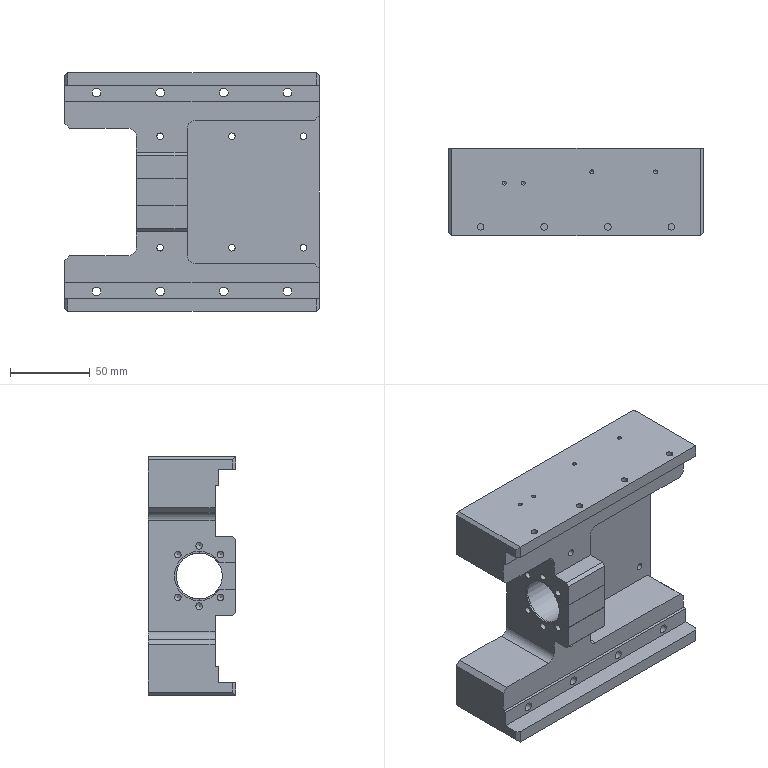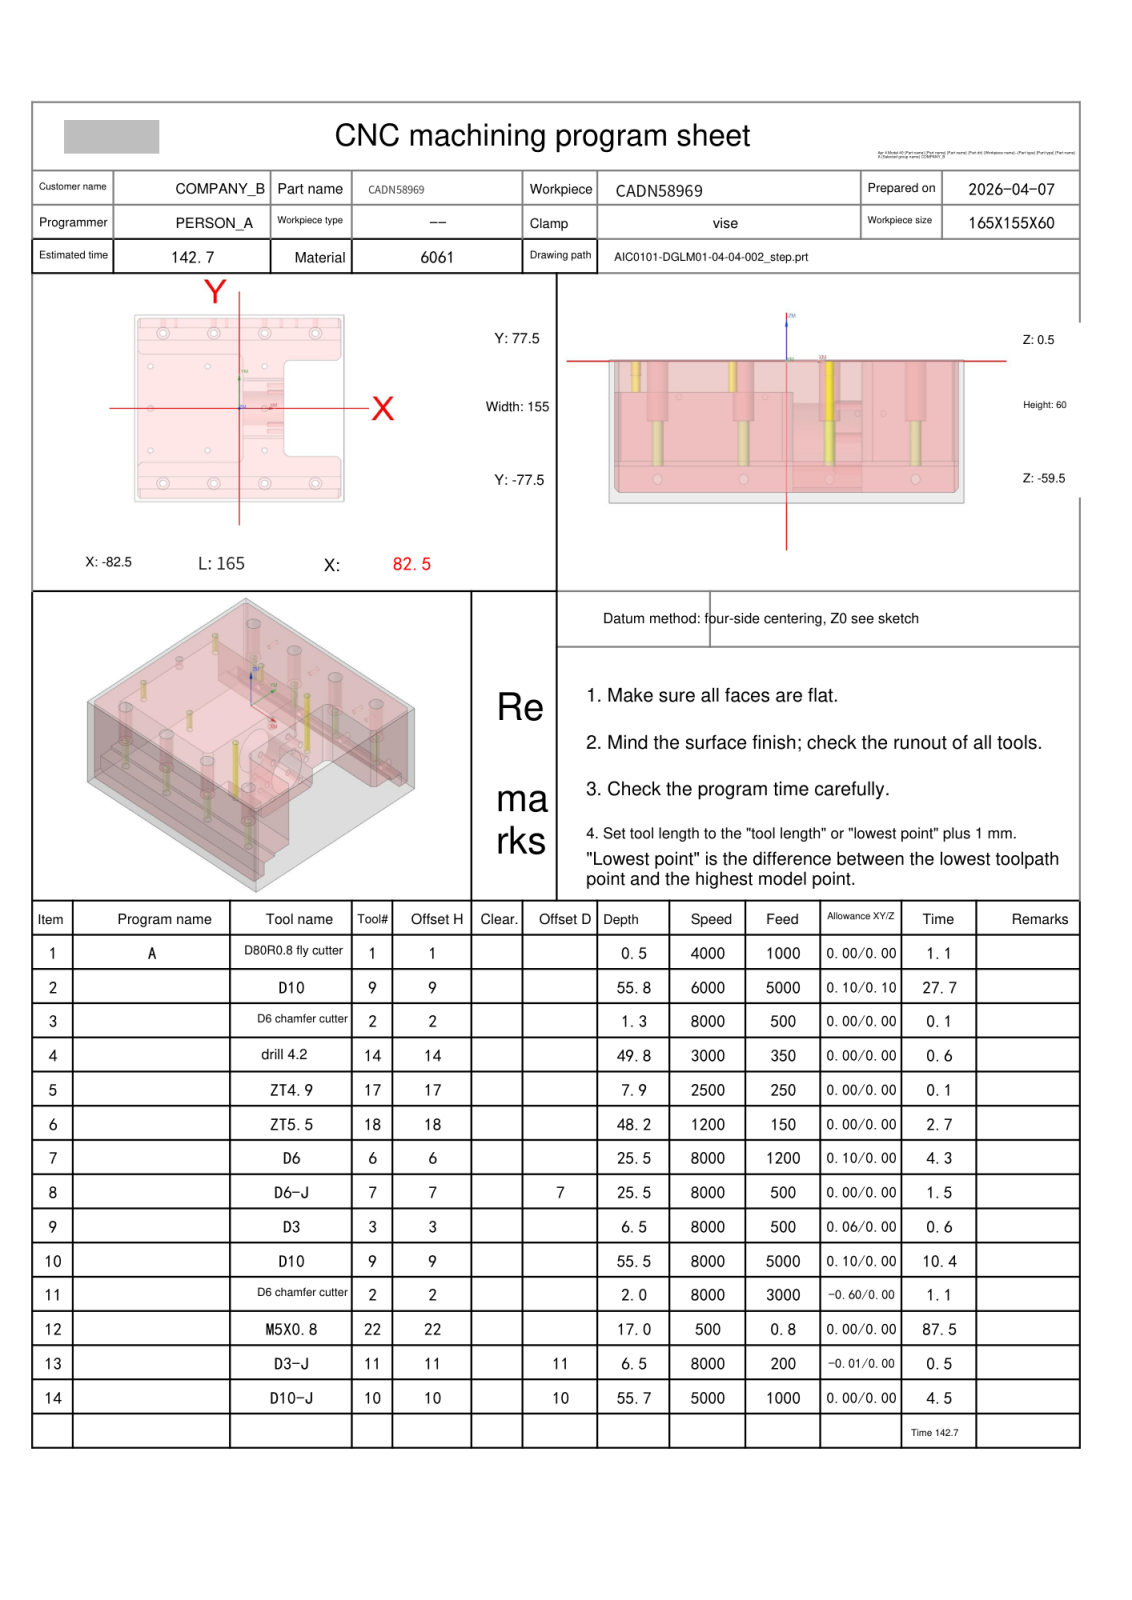NC program | NX | posted by the shop | part box 160 x 55 x 150 mm
Lines 13089 to 13884 of 15707:
N10 T09 M06
(D10  D=10. R=0. H=09 ce=0.10 di=0.00)
G00 G90 G54 X0.0 Y80.1 M03 S8000
G43 H09 Z20.
M08
Z.5
G01 X78. Z.415 F5000.
G02 X81.606 Y78.606 Z.411 I0.0 J-5.1
G01 X83.606 Y76.606 Z.408
G02 X85.1 Y73. Z.403 I-3.606 J-3.606
G01 Y43. Z.371
G02 X83.606 Y39.394 Z.366 I-5.1 J0.0
G01 X80.606 Y36.394 Z.362
G02 X77. Y34.9 Z.358 I-3.606 J3.606
G01 X40.1 Z.317
Y-34.9 Z.242
X77. Z.201
G02 X80.606 Y-36.394 Z.197 I0.0 J-5.1
G01 X83.606 Y-39.394 Z.192
G02 X85.1 Y-43. Z.188 I-3.606 J-3.606
G01 Y-73. Z.156
G02 X83.606 Y-76.606 Z.151 I-5.1 J0.0
G01 X81.606 Y-78.606 Z.148
G02 X78. Y-80.1 Z.144 I-3.606 J3.606
G01 X-78. Z-.026
G02 X-81.606 Y-78.606 Z-.03 I0.0 J5.1
G01 X-83.606 Y-76.606 Z-.033
G02 X-85.1 Y-73. Z-.038 I3.606 J3.606
G01 Y73. Z-.196
G02 X-83.606 Y76.606 Z-.201 I5.1 J0.0
G01 X-81.606 Y78.606 Z-.204
G02 X-78. Y80.1 Z-.208 I3.606 J-3.606
G01 X78. Z-.378
G02 X81.606 Y78.606 Z-.382 I0.0 J-5.1
G01 X83.606 Y76.606 Z-.385
G02 X85.1 Y73. Z-.389 I-3.606 J-3.606
G01 Y43. Z-.422
G02 X83.606 Y39.394 Z-.426 I-5.1 J0.0
G01 X80.606 Y36.394 Z-.431
G02 X77. Y34.9 Z-.435 I-3.606 J3.606
G01 X40.1 Z-.475
Y-34.9 Z-.551
X77. Z-.591
G02 X80.606 Y-36.394 Z-.596 I0.0 J-5.1
G01 X83.606 Y-39.394 Z-.6
G02 X85.1 Y-43. Z-.605 I-3.606 J-3.606
G01 Y-73. Z-.637
G02 X83.606 Y-76.606 Z-.642 I-5.1 J0.0
G01 X81.606 Y-78.606 Z-.645
G02 X78. Y-80.1 Z-.649 I-3.606 J3.606
G01 X-78. Z-.819
G02 X-81.606 Y-78.606 Z-.823 I0.0 J5.1
G01 X-83.606 Y-76.606 Z-.826
G02 X-85.1 Y-73. Z-.83 I3.606 J3.606
G01 Y73. Z-.989
G02 X-83.606 Y76.606 Z-.994 I5.1 J0.0
G01 X-81.606 Y78.606 Z-.997
G02 X-78. Y80.1 Z-1.001 I3.606 J-3.606
G01 X78. Z-1.17
G02 X81.606 Y78.606 Z-1.175 I0.0 J-5.1
G01 X83.606 Y76.606 Z-1.178
G02 X85.1 Y73. Z-1.182 I-3.606 J-3.606
G01 Y43. Z-1.215
G02 X83.606 Y39.394 Z-1.219 I-5.1 J0.0
G01 X80.606 Y36.394 Z-1.224
G02 X77. Y34.9 Z-1.228 I-3.606 J3.606
G01 X40.1 Z-1.268
Y-34.9 Z-1.344
X77. Z-1.384
G02 X80.606 Y-36.394 Z-1.389 I0.0 J-5.1
G01 X83.606 Y-39.394 Z-1.393
G02 X85.1 Y-43. Z-1.398 I-3.606 J-3.606
G01 Y-73. Z-1.43
G02 X83.606 Y-76.606 Z-1.435 I-5.1 J0.0
G01 X81.606 Y-78.606 Z-1.438
G02 X78. Y-80.1 Z-1.442 I-3.606 J3.606
G01 X-78. Z-1.612
G02 X-81.606 Y-78.606 Z-1.616 I0.0 J5.1
G01 X-83.606 Y-76.606 Z-1.619
G02 X-85.1 Y-73. Z-1.623 I3.606 J3.606
G01 Y73. Z-1.782
G02 X-83.606 Y76.606 Z-1.786 I5.1 J0.0
G01 X-81.606 Y78.606 Z-1.789
G02 X-78. Y80.1 Z-1.794 I3.606 J-3.606
G01 X78. Z-1.963
G02 X81.606 Y78.606 Z-1.968 I0.0 J-5.1
G01 X83.606 Y76.606 Z-1.971
G02 X85.1 Y73. Z-1.975 I-3.606 J-3.606
G01 Y43. Z-2.008
G02 X83.606 Y39.394 Z-2.012 I-5.1 J0.0
G01 X80.606 Y36.394 Z-2.017
G02 X77. Y34.9 Z-2.021 I-3.606 J3.606
G01 X40.1 Z-2.061
Y-34.9 Z-2.137
X77. Z-2.177
G02 X80.606 Y-36.394 Z-2.181 I0.0 J-5.1
G01 X83.606 Y-39.394 Z-2.186
G02 X85.1 Y-43. Z-2.19 I-3.606 J-3.606
G01 Y-73. Z-2.223
G02 X83.606 Y-76.606 Z-2.227 I-5.1 J0.0
G01 X81.606 Y-78.606 Z-2.23
G02 X78. Y-80.1 Z-2.235 I-3.606 J3.606
G01 X-78. Z-2.404
G02 X-81.606 Y-78.606 Z-2.409 I0.0 J5.1
G01 X-83.606 Y-76.606 Z-2.412
G02 X-85.1 Y-73. Z-2.416 I3.606 J3.606
G01 Y73. Z-2.575
G02 X-83.606 Y76.606 Z-2.579 I5.1 J0.0
G01 X-81.606 Y78.606 Z-2.582
G02 X-78. Y80.1 Z-2.587 I3.606 J-3.606
G01 X78. Z-2.756
G02 X81.606 Y78.606 Z-2.761 I0.0 J-5.1
G01 X83.606 Y76.606 Z-2.764
G02 X85.1 Y73. Z-2.768 I-3.606 J-3.606
G01 Y43. Z-2.801
G02 X83.606 Y39.394 Z-2.805 I-5.1 J0.0
G01 X80.606 Y36.394 Z-2.81
G02 X77. Y34.9 Z-2.814 I-3.606 J3.606
G01 X40.1 Z-2.854
Y-34.9 Z-2.93
X77. Z-2.97
G02 X80.606 Y-36.394 Z-2.974 I0.0 J-5.1
G01 X83.606 Y-39.394 Z-2.979
G02 X85.1 Y-43. Z-2.983 I-3.606 J-3.606
G01 Y-73. Z-3.016
G02 X83.606 Y-76.606 Z-3.02 I-5.1 J0.0
G01 X81.606 Y-78.606 Z-3.023
G02 X78. Y-80.1 Z-3.028 I-3.606 J3.606
G01 X-78. Z-3.197
G02 X-81.606 Y-78.606 Z-3.202 I0.0 J5.1
G01 X-83.606 Y-76.606 Z-3.205
G02 X-85.1 Y-73. Z-3.209 I3.606 J3.606
G01 Y73. Z-3.368
G02 X-83.606 Y76.606 Z-3.372 I5.1 J0.0
G01 X-81.606 Y78.606 Z-3.375
G02 X-78. Y80.1 Z-3.38 I3.606 J-3.606
G01 X78. Z-3.549
G02 X81.606 Y78.606 Z-3.553 I0.0 J-5.1
G01 X83.606 Y76.606 Z-3.556
G02 X85.1 Y73. Z-3.561 I-3.606 J-3.606
G01 Y43. Z-3.593
G02 X83.606 Y39.394 Z-3.598 I-5.1 J0.0
G01 X80.606 Y36.394 Z-3.602
G02 X77. Y34.9 Z-3.607 I-3.606 J3.606
G01 X40.1 Z-3.647
Y-34.9 Z-3.723
X77. Z-3.763
G02 X80.606 Y-36.394 Z-3.767 I0.0 J-5.1
G01 X83.606 Y-39.394 Z-3.772
G02 X85.1 Y-43. Z-3.776 I-3.606 J-3.606
G01 Y-73. Z-3.809
G02 X83.606 Y-76.606 Z-3.813 I-5.1 J0.0
G01 X81.606 Y-78.606 Z-3.816
G02 X78. Y-80.1 Z-3.821 I-3.606 J3.606
G01 X-78. Z-3.99
G02 X-81.606 Y-78.606 Z-3.994 I0.0 J5.1
G01 X-83.606 Y-76.606 Z-3.998
G02 X-85.1 Y-73. Z-4.002 I3.606 J3.606
G01 Y73. Z-4.161
G02 X-83.606 Y76.606 Z-4.165 I5.1 J0.0
G01 X-81.606 Y78.606 Z-4.168
G02 X-78. Y80.1 Z-4.172 I3.606 J-3.606
G01 X78. Z-4.342
G02 X81.606 Y78.606 Z-4.346 I0.0 J-5.1
G01 X83.606 Y76.606 Z-4.349
G02 X85.1 Y73. Z-4.354 I-3.606 J-3.606
G01 Y43. Z-4.386
G02 X83.606 Y39.394 Z-4.391 I-5.1 J0.0
G01 X80.606 Y36.394 Z-4.395
G02 X77. Y34.9 Z-4.4 I-3.606 J3.606
G01 X40.1 Z-4.44
Y-34.9 Z-4.516
X77. Z-4.556
G02 X80.606 Y-36.394 Z-4.56 I0.0 J-5.1
G01 X83.606 Y-39.394 Z-4.565
G02 X85.1 Y-43. Z-4.569 I-3.606 J-3.606
G01 Y-73. Z-4.602
G02 X83.606 Y-76.606 Z-4.606 I-5.1 J0.0
G01 X81.606 Y-78.606 Z-4.609
G02 X78. Y-80.1 Z-4.613 I-3.606 J3.606
G01 X-78. Z-4.783
G02 X-81.606 Y-78.606 Z-4.787 I0.0 J5.1
G01 X-83.606 Y-76.606 Z-4.79
G02 X-85.1 Y-73. Z-4.795 I3.606 J3.606
G01 Y73. Z-4.953
G02 X-83.606 Y76.606 Z-4.958 I5.1 J0.0
G01 X-81.606 Y78.606 Z-4.961
G02 X-78. Y80.1 Z-4.965 I3.606 J-3.606
G01 X78. Z-5.135
G02 X81.606 Y78.606 Z-5.139 I0.0 J-5.1
G01 X83.606 Y76.606 Z-5.142
G02 X85.1 Y73. Z-5.147 I-3.606 J-3.606
G01 Y43. Z-5.179
G02 X83.606 Y39.394 Z-5.184 I-5.1 J0.0
G01 X80.606 Y36.394 Z-5.188
G02 X77. Y34.9 Z-5.192 I-3.606 J3.606
G01 X40.1 Z-5.233
Y-34.9 Z-5.308
X77. Z-5.349
G02 X80.606 Y-36.394 Z-5.353 I0.0 J-5.1
G01 X83.606 Y-39.394 Z-5.358
G02 X85.1 Y-43. Z-5.362 I-3.606 J-3.606
G01 Y-73. Z-5.394
G02 X83.606 Y-76.606 Z-5.399 I-5.1 J0.0
G01 X81.606 Y-78.606 Z-5.402
G02 X78. Y-80.1 Z-5.406 I-3.606 J3.606
G01 X-78. Z-5.576
G02 X-81.606 Y-78.606 Z-5.58 I0.0 J5.1
G01 X-83.606 Y-76.606 Z-5.583
G02 X-85.1 Y-73. Z-5.588 I3.606 J3.606
G01 Y73. Z-5.746
G02 X-83.606 Y76.606 Z-5.751 I5.1 J0.0
G01 X-81.606 Y78.606 Z-5.754
G02 X-78. Y80.1 Z-5.758 I3.606 J-3.606
G01 X78. Z-5.928
G02 X81.606 Y78.606 Z-5.932 I0.0 J-5.1
G01 X83.606 Y76.606 Z-5.935
G02 X85.1 Y73. Z-5.939 I-3.606 J-3.606
G01 Y43. Z-5.972
G02 X83.606 Y39.394 Z-5.976 I-5.1 J0.0
G01 X80.606 Y36.394 Z-5.981
G02 X77. Y34.9 Z-5.985 I-3.606 J3.606
G01 X40.1 Z-6.025
Y-34.9 Z-6.101
X77. Z-6.141
G02 X80.606 Y-36.394 Z-6.146 I0.0 J-5.1
G01 X83.606 Y-39.394 Z-6.15
G02 X85.1 Y-43. Z-6.155 I-3.606 J-3.606
G01 Y-73. Z-6.187
G02 X83.606 Y-76.606 Z-6.192 I-5.1 J0.0
G01 X81.606 Y-78.606 Z-6.195
G02 X78. Y-80.1 Z-6.199 I-3.606 J3.606
G01 X-78. Z-6.369
G02 X-81.606 Y-78.606 Z-6.373 I0.0 J5.1
G01 X-83.606 Y-76.606 Z-6.376
G02 X-85.1 Y-73. Z-6.38 I3.606 J3.606
G01 Y73. Z-6.539
G02 X-83.606 Y76.606 Z-6.544 I5.1 J0.0
G01 X-81.606 Y78.606 Z-6.547
G02 X-78. Y80.1 Z-6.551 I3.606 J-3.606
G01 X78. Z-6.72
G02 X81.606 Y78.606 Z-6.725 I0.0 J-5.1
G01 X83.606 Y76.606 Z-6.728
G02 X85.1 Y73. Z-6.732 I-3.606 J-3.606
G01 Y43. Z-6.765
G02 X83.606 Y39.394 Z-6.769 I-5.1 J0.0
G01 X80.606 Y36.394 Z-6.774
G02 X77. Y34.9 Z-6.778 I-3.606 J3.606
G01 X40.1 Z-6.818
Y-34.9 Z-6.894
X77. Z-6.934
G02 X80.606 Y-36.394 Z-6.939 I0.0 J-5.1
G01 X83.606 Y-39.394 Z-6.943
G02 X85.1 Y-43. Z-6.948 I-3.606 J-3.606
G01 Y-73. Z-6.98
G02 X83.606 Y-76.606 Z-6.985 I-5.1 J0.0
G01 X81.606 Y-78.606 Z-6.988
G02 X78. Y-80.1 Z-6.992 I-3.606 J3.606
G01 X-78. Z-7.162
G02 X-81.606 Y-78.606 Z-7.166 I0.0 J5.1
G01 X-83.606 Y-76.606 Z-7.169
G02 X-85.1 Y-73. Z-7.173 I3.606 J3.606
G01 Y73. Z-7.332
G02 X-83.606 Y76.606 Z-7.336 I5.1 J0.0
G01 X-81.606 Y78.606 Z-7.339
G02 X-78. Y80.1 Z-7.344 I3.606 J-3.606
G01 X78. Z-7.513
G02 X81.606 Y78.606 Z-7.518 I0.0 J-5.1
G01 X83.606 Y76.606 Z-7.521
G02 X85.1 Y73. Z-7.525 I-3.606 J-3.606
G01 Y43. Z-7.558
G02 X83.606 Y39.394 Z-7.562 I-5.1 J0.0
G01 X80.606 Y36.394 Z-7.567
G02 X77. Y34.9 Z-7.571 I-3.606 J3.606
G01 X40.1 Z-7.611
Y-34.9 Z-7.687
X77. Z-7.727
G02 X80.606 Y-36.394 Z-7.731 I0.0 J-5.1
G01 X83.606 Y-39.394 Z-7.736
G02 X85.1 Y-43. Z-7.74 I-3.606 J-3.606
G01 Y-73. Z-7.773
G02 X83.606 Y-76.606 Z-7.777 I-5.1 J0.0
G01 X81.606 Y-78.606 Z-7.78
G02 X78. Y-80.1 Z-7.785 I-3.606 J3.606
G01 X-78. Z-7.954
G02 X-81.606 Y-78.606 Z-7.959 I0.0 J5.1
G01 X-83.606 Y-76.606 Z-7.962
G02 X-85.1 Y-73. Z-7.966 I3.606 J3.606
G01 Y73. Z-8.125
G02 X-83.606 Y76.606 Z-8.129 I5.1 J0.0
G01 X-81.606 Y78.606 Z-8.132
G02 X-78. Y80.1 Z-8.137 I3.606 J-3.606
G01 X78. Z-8.306
G02 X81.606 Y78.606 Z-8.311 I0.0 J-5.1
G01 X83.606 Y76.606 Z-8.314
G02 X85.1 Y73. Z-8.318 I-3.606 J-3.606
G01 Y43. Z-8.351
G02 X83.606 Y39.394 Z-8.355 I-5.1 J0.0
G01 X80.606 Y36.394 Z-8.36
G02 X77. Y34.9 Z-8.364 I-3.606 J3.606
G01 X40.1 Z-8.404
Y-34.9 Z-8.48
X77. Z-8.52
G02 X80.606 Y-36.394 Z-8.524 I0.0 J-5.1
G01 X83.606 Y-39.394 Z-8.529
G02 X85.1 Y-43. Z-8.533 I-3.606 J-3.606
G01 Y-73. Z-8.566
G02 X83.606 Y-76.606 Z-8.57 I-5.1 J0.0
G01 X81.606 Y-78.606 Z-8.573
G02 X78. Y-80.1 Z-8.578 I-3.606 J3.606
G01 X-78. Z-8.747
G02 X-81.606 Y-78.606 Z-8.752 I0.0 J5.1
G01 X-83.606 Y-76.606 Z-8.755
G02 X-85.1 Y-73. Z-8.759 I3.606 J3.606
G01 Y73. Z-8.918
G02 X-83.606 Y76.606 Z-8.922 I5.1 J0.0
G01 X-81.606 Y78.606 Z-8.925
G02 X-78. Y80.1 Z-8.93 I3.606 J-3.606
G01 X78. Z-9.099
G02 X81.606 Y78.606 Z-9.103 I0.0 J-5.1
G01 X83.606 Y76.606 Z-9.106
G02 X85.1 Y73. Z-9.111 I-3.606 J-3.606
G01 Y43. Z-9.143
G02 X83.606 Y39.394 Z-9.148 I-5.1 J0.0
G01 X80.606 Y36.394 Z-9.152
G02 X77. Y34.9 Z-9.157 I-3.606 J3.606
G01 X40.1 Z-9.197
Y-34.9 Z-9.273
X77. Z-9.313
G02 X80.606 Y-36.394 Z-9.317 I0.0 J-5.1
G01 X83.606 Y-39.394 Z-9.322
G02 X85.1 Y-43. Z-9.326 I-3.606 J-3.606
G01 Y-73. Z-9.359
G02 X83.606 Y-76.606 Z-9.363 I-5.1 J0.0
G01 X81.606 Y-78.606 Z-9.366
G02 X78. Y-80.1 Z-9.371 I-3.606 J3.606
G01 X-78. Z-9.54
G02 X-81.606 Y-78.606 Z-9.544 I0.0 J5.1
G01 X-83.606 Y-76.606 Z-9.548
G02 X-85.1 Y-73. Z-9.552 I3.606 J3.606
G01 Y73. Z-9.711
G02 X-83.606 Y76.606 Z-9.715 I5.1 J0.0
G01 X-81.606 Y78.606 Z-9.718
G02 X-78. Y80.1 Z-9.722 I3.606 J-3.606
G01 X78. Z-9.892
G02 X81.606 Y78.606 Z-9.896 I0.0 J-5.1
G01 X83.606 Y76.606 Z-9.899
G02 X85.1 Y73. Z-9.904 I-3.606 J-3.606
G01 Y43. Z-9.936
G02 X83.606 Y39.394 Z-9.941 I-5.1 J0.0
G01 X80.606 Y36.394 Z-9.945
G02 X77. Y34.9 Z-9.95 I-3.606 J3.606
G01 X40.1 Z-9.99
Y-34.9 Z-10.066
X77. Z-10.106
G02 X80.606 Y-36.394 Z-10.11 I0.0 J-5.1
G01 X83.606 Y-39.394 Z-10.115
G02 X85.1 Y-43. Z-10.119 I-3.606 J-3.606
G01 Y-73. Z-10.152
G02 X83.606 Y-76.606 Z-10.156 I-5.1 J0.0
G01 X81.606 Y-78.606 Z-10.159
G02 X78. Y-80.1 Z-10.163 I-3.606 J3.606
G01 X-78. Z-10.333
G02 X-81.606 Y-78.606 Z-10.337 I0.0 J5.1
G01 X-83.606 Y-76.606 Z-10.34
G02 X-85.1 Y-73. Z-10.345 I3.606 J3.606
G01 Y73. Z-10.503
G02 X-83.606 Y76.606 Z-10.508 I5.1 J0.0
G01 X-81.606 Y78.606 Z-10.511
G02 X-78. Y80.1 Z-10.515 I3.606 J-3.606
G01 X78. Z-10.685
G02 X81.606 Y78.606 Z-10.689 I0.0 J-5.1
G01 X83.606 Y76.606 Z-10.692
G02 X85.1 Y73. Z-10.697 I-3.606 J-3.606
G01 Y43. Z-10.729
G02 X83.606 Y39.394 Z-10.734 I-5.1 J0.0
G01 X80.606 Y36.394 Z-10.738
G02 X77. Y34.9 Z-10.742 I-3.606 J3.606
G01 X40.1 Z-10.783
Y-34.9 Z-10.858
X77. Z-10.899
G02 X80.606 Y-36.394 Z-10.903 I0.0 J-5.1
G01 X83.606 Y-39.394 Z-10.908
G02 X85.1 Y-43. Z-10.912 I-3.606 J-3.606
G01 Y-73. Z-10.944
G02 X83.606 Y-76.606 Z-10.949 I-5.1 J0.0
G01 X81.606 Y-78.606 Z-10.952
G02 X78. Y-80.1 Z-10.956 I-3.606 J3.606
G01 X-78. Z-11.126
G02 X-81.606 Y-78.606 Z-11.13 I0.0 J5.1
G01 X-83.606 Y-76.606 Z-11.133
G02 X-85.1 Y-73. Z-11.138 I3.606 J3.606
G01 Y73. Z-11.296
G02 X-83.606 Y76.606 Z-11.301 I5.1 J0.0
G01 X-81.606 Y78.606 Z-11.304
G02 X-78. Y80.1 Z-11.308 I3.606 J-3.606
G01 X78. Z-11.478
G02 X81.606 Y78.606 Z-11.482 I0.0 J-5.1
G01 X83.606 Y76.606 Z-11.485
G02 X85.1 Y73. Z-11.489 I-3.606 J-3.606
G01 Y43. Z-11.522
G02 X83.606 Y39.394 Z-11.526 I-5.1 J0.0
G01 X80.606 Y36.394 Z-11.531
G02 X77. Y34.9 Z-11.535 I-3.606 J3.606
G01 X40.1 Z-11.575
Y-34.9 Z-11.651
X77. Z-11.691
G02 X80.606 Y-36.394 Z-11.696 I0.0 J-5.1
G01 X83.606 Y-39.394 Z-11.7
G02 X85.1 Y-43. Z-11.705 I-3.606 J-3.606
G01 Y-73. Z-11.737
G02 X83.606 Y-76.606 Z-11.742 I-5.1 J0.0
G01 X81.606 Y-78.606 Z-11.745
G02 X78. Y-80.1 Z-11.749 I-3.606 J3.606
G01 X-78. Z-11.919
G02 X-81.606 Y-78.606 Z-11.923 I0.0 J5.1
G01 X-83.606 Y-76.606 Z-11.926
G02 X-85.1 Y-73. Z-11.93 I3.606 J3.606
G01 Y73. Z-12.089
G02 X-83.606 Y76.606 Z-12.094 I5.1 J0.0
G01 X-81.606 Y78.606 Z-12.097
G02 X-78. Y80.1 Z-12.101 I3.606 J-3.606
G01 X78. Z-12.27
G02 X81.606 Y78.606 Z-12.275 I0.0 J-5.1
G01 X83.606 Y76.606 Z-12.278
G02 X85.1 Y73. Z-12.282 I-3.606 J-3.606
G01 Y43. Z-12.315
G02 X83.606 Y39.394 Z-12.319 I-5.1 J0.0
G01 X80.606 Y36.394 Z-12.324
G02 X77. Y34.9 Z-12.328 I-3.606 J3.606
G01 X40.1 Z-12.368
Y-34.9 Z-12.444
X77. Z-12.484
G02 X80.606 Y-36.394 Z-12.489 I0.0 J-5.1
G01 X83.606 Y-39.394 Z-12.493
G02 X85.1 Y-43. Z-12.498 I-3.606 J-3.606
G01 Y-73. Z-12.53
G02 X83.606 Y-76.606 Z-12.535 I-5.1 J0.0
G01 X81.606 Y-78.606 Z-12.538
G02 X78. Y-80.1 Z-12.542 I-3.606 J3.606
G01 X-78. Z-12.712
G02 X-81.606 Y-78.606 Z-12.716 I0.0 J5.1
G01 X-83.606 Y-76.606 Z-12.719
G02 X-85.1 Y-73. Z-12.723 I3.606 J3.606
G01 Y73. Z-12.882
G02 X-83.606 Y76.606 Z-12.886 I5.1 J0.0
G01 X-81.606 Y78.606 Z-12.889
G02 X-78. Y80.1 Z-12.894 I3.606 J-3.606
G01 X78. Z-13.063
G02 X81.606 Y78.606 Z-13.068 I0.0 J-5.1
G01 X83.606 Y76.606 Z-13.071
G02 X85.1 Y73. Z-13.075 I-3.606 J-3.606
G01 Y43. Z-13.108
G02 X83.606 Y39.394 Z-13.112 I-5.1 J0.0
G01 X80.606 Y36.394 Z-13.117
G02 X77. Y34.9 Z-13.121 I-3.606 J3.606
G01 X40.1 Z-13.161
Y-34.9 Z-13.237
X77. Z-13.277
G02 X80.606 Y-36.394 Z-13.281 I0.0 J-5.1
G01 X83.606 Y-39.394 Z-13.286
G02 X85.1 Y-43. Z-13.29 I-3.606 J-3.606
G01 Y-73. Z-13.323
G02 X83.606 Y-76.606 Z-13.327 I-5.1 J0.0
G01 X81.606 Y-78.606 Z-13.33
G02 X78. Y-80.1 Z-13.335 I-3.606 J3.606
G01 X-78. Z-13.504
G02 X-81.606 Y-78.606 Z-13.509 I0.0 J5.1
G01 X-83.606 Y-76.606 Z-13.512
G02 X-85.1 Y-73. Z-13.516 I3.606 J3.606
G01 Y73. Z-13.675
G02 X-83.606 Y76.606 Z-13.679 I5.1 J0.0
G01 X-81.606 Y78.606 Z-13.682
G02 X-78. Y80.1 Z-13.687 I3.606 J-3.606
G01 X78. Z-13.856
G02 X81.606 Y78.606 Z-13.861 I0.0 J-5.1
G01 X83.606 Y76.606 Z-13.864
G02 X85.1 Y73. Z-13.868 I-3.606 J-3.606
G01 Y43. Z-13.901
G02 X83.606 Y39.394 Z-13.905 I-5.1 J0.0
G01 X80.606 Y36.394 Z-13.91
G02 X77. Y34.9 Z-13.914 I-3.606 J3.606
G01 X40.1 Z-13.954
Y-34.9 Z-14.03
X77. Z-14.07
G02 X80.606 Y-36.394 Z-14.074 I0.0 J-5.1
G01 X83.606 Y-39.394 Z-14.079
G02 X85.1 Y-43. Z-14.083 I-3.606 J-3.606
G01 Y-73. Z-14.116
G02 X83.606 Y-76.606 Z-14.12 I-5.1 J0.0
G01 X81.606 Y-78.606 Z-14.123
G02 X78. Y-80.1 Z-14.128 I-3.606 J3.606
G01 X-78. Z-14.297
G02 X-81.606 Y-78.606 Z-14.302 I0.0 J5.1
G01 X-83.606 Y-76.606 Z-14.305
G02 X-85.1 Y-73. Z-14.309 I3.606 J3.606
G01 Y73. Z-14.468
G02 X-83.606 Y76.606 Z-14.472 I5.1 J0.0
G01 X-81.606 Y78.606 Z-14.475
G02 X-78. Y80.1 Z-14.48 I3.606 J-3.606
G01 X78. Z-14.649
G02 X81.606 Y78.606 Z-14.653 I0.0 J-5.1
G01 X83.606 Y76.606 Z-14.656
G02 X85.1 Y73. Z-14.661 I-3.606 J-3.606
G01 Y43. Z-14.693
G02 X83.606 Y39.394 Z-14.698 I-5.1 J0.0
G01 X80.606 Y36.394 Z-14.702
G02 X77. Y34.9 Z-14.707 I-3.606 J3.606
G01 X40.1 Z-14.747
Y-34.9 Z-14.823
X77. Z-14.863
G02 X80.606 Y-36.394 Z-14.867 I0.0 J-5.1
G01 X83.606 Y-39.394 Z-14.872
G02 X85.1 Y-43. Z-14.876 I-3.606 J-3.606
G01 Y-73. Z-14.909
G02 X83.606 Y-76.606 Z-14.913 I-5.1 J0.0
G01 X81.606 Y-78.606 Z-14.916
G02 X78. Y-80.1 Z-14.921 I-3.606 J3.606
G01 X-78. Z-15.09
G02 X-81.606 Y-78.606 Z-15.094 I0.0 J5.1
G01 X-83.606 Y-76.606 Z-15.098
G02 X-85.1 Y-73. Z-15.102 I3.606 J3.606
G01 Y73. Z-15.261
G02 X-83.606 Y76.606 Z-15.265 I5.1 J0.0
G01 X-81.606 Y78.606 Z-15.268
G02 X-78. Y80.1 Z-15.272 I3.606 J-3.606
G01 X78. Z-15.442
G02 X81.606 Y78.606 Z-15.446 I0.0 J-5.1
G01 X83.606 Y76.606 Z-15.449
G02 X85.1 Y73. Z-15.454 I-3.606 J-3.606
G01 Y43. Z-15.486
G02 X83.606 Y39.394 Z-15.491 I-5.1 J0.0
G01 X80.606 Y36.394 Z-15.495
G02 X77. Y34.9 Z-15.5 I-3.606 J3.606
G01 X40.1 Z-15.54
Y-34.9 Z-15.616
X77. Z-15.656
G02 X80.606 Y-36.394 Z-15.66 I0.0 J-5.1
G01 X83.606 Y-39.394 Z-15.665
G02 X85.1 Y-43. Z-15.669 I-3.606 J-3.606
G01 Y-73. Z-15.702
G02 X83.606 Y-76.606 Z-15.706 I-5.1 J0.0
G01 X81.606 Y-78.606 Z-15.709
G02 X78. Y-80.1 Z-15.713 I-3.606 J3.606
G01 X-78. Z-15.883
G02 X-81.606 Y-78.606 Z-15.887 I0.0 J5.1
G01 X-83.606 Y-76.606 Z-15.89
G02 X-85.1 Y-73. Z-15.895 I3.606 J3.606
G01 Y73. Z-16.053
G02 X-83.606 Y76.606 Z-16.058 I5.1 J0.0
G01 X-81.606 Y78.606 Z-16.061
G02 X-78. Y80.1 Z-16.065 I3.606 J-3.606
G01 X78. Z-16.235
G02 X81.606 Y78.606 Z-16.239 I0.0 J-5.1
G01 X83.606 Y76.606 Z-16.242
G02 X85.1 Y73. Z-16.247 I-3.606 J-3.606
G01 Y43. Z-16.279
G02 X83.606 Y39.394 Z-16.284 I-5.1 J0.0
G01 X80.606 Y36.394 Z-16.288
G02 X77. Y34.9 Z-16.292 I-3.606 J3.606
G01 X40.1 Z-16.333
Y-34.9 Z-16.408
X77. Z-16.449
G02 X80.606 Y-36.394 Z-16.453 I0.0 J-5.1
G01 X83.606 Y-39.394 Z-16.458
G02 X85.1 Y-43. Z-16.462 I-3.606 J-3.606
G01 Y-73. Z-16.494
G02 X83.606 Y-76.606 Z-16.499 I-5.1 J0.0
G01 X81.606 Y-78.606 Z-16.502
G02 X78. Y-80.1 Z-16.506 I-3.606 J3.606
G01 X-78. Z-16.676
G02 X-81.606 Y-78.606 Z-16.68 I0.0 J5.1
G01 X-83.606 Y-76.606 Z-16.683
G02 X-85.1 Y-73. Z-16.688 I3.606 J3.606
G01 Y73. Z-16.846
G02 X-83.606 Y76.606 Z-16.851 I5.1 J0.0
G01 X-81.606 Y78.606 Z-16.854
G02 X-78. Y80.1 Z-16.858 I3.606 J-3.606
G01 X78. Z-17.028
G02 X81.606 Y78.606 Z-17.032 I0.0 J-5.1
G01 X83.606 Y76.606 Z-17.035
G02 X85.1 Y73. Z-17.039 I-3.606 J-3.606
G01 Y43. Z-17.072
G02 X83.606 Y39.394 Z-17.076 I-5.1 J0.0
G01 X80.606 Y36.394 Z-17.081
G02 X77. Y34.9 Z-17.085 I-3.606 J3.606
G01 X40.1 Z-17.125
Y-34.9 Z-17.201
X77. Z-17.241
G02 X80.606 Y-36.394 Z-17.246 I0.0 J-5.1
G01 X83.606 Y-39.394 Z-17.25
G02 X85.1 Y-43. Z-17.255 I-3.606 J-3.606
G01 Y-73. Z-17.287
G02 X83.606 Y-76.606 Z-17.292 I-5.1 J0.0
G01 X81.606 Y-78.606 Z-17.295
G02 X78. Y-80.1 Z-17.299 I-3.606 J3.606
G01 X-78. Z-17.469
G02 X-81.606 Y-78.606 Z-17.473 I0.0 J5.1
G01 X-83.606 Y-76.606 Z-17.476
G02 X-85.1 Y-73. Z-17.48 I3.606 J3.606
G01 Y73. Z-17.639
G02 X-83.606 Y76.606 Z-17.644 I5.1 J0.0
G01 X-81.606 Y78.606 Z-17.647
G02 X-78. Y80.1 Z-17.651 I3.606 J-3.606
G01 X78. Z-17.82
G02 X81.606 Y78.606 Z-17.825 I0.0 J-5.1
G01 X83.606 Y76.606 Z-17.828
G02 X85.1 Y73. Z-17.832 I-3.606 J-3.606
G01 Y43. Z-17.865
G02 X83.606 Y39.394 Z-17.869 I-5.1 J0.0
G01 X80.606 Y36.394 Z-17.874
G02 X77. Y34.9 Z-17.878 I-3.606 J3.606
G01 X40.1 Z-17.918
Y-34.9 Z-17.994
X77. Z-18.034
G02 X80.606 Y-36.394 Z-18.039 I0.0 J-5.1
G01 X83.606 Y-39.394 Z-18.043
G02 X85.1 Y-43. Z-18.048 I-3.606 J-3.606
G01 Y-73. Z-18.08
G02 X83.606 Y-76.606 Z-18.085 I-5.1 J0.0
G01 X81.606 Y-78.606 Z-18.088
G02 X78. Y-80.1 Z-18.092 I-3.606 J3.606
G01 X-78. Z-18.262
G02 X-81.606 Y-78.606 Z-18.266 I0.0 J5.1
G01 X-83.606 Y-76.606 Z-18.269
G02 X-85.1 Y-73. Z-18.273 I3.606 J3.606
G01 Y73. Z-18.432
G02 X-83.606 Y76.606 Z-18.436 I5.1 J0.0
G01 X-81.606 Y78.606 Z-18.439
G02 X-78. Y80.1 Z-18.444 I3.606 J-3.606
G01 X78. Z-18.613
G02 X81.606 Y78.606 Z-18.618 I0.0 J-5.1
G01 X83.606 Y76.606 Z-18.621
G02 X85.1 Y73. Z-18.625 I-3.606 J-3.606
G01 Y43. Z-18.658
G02 X83.606 Y39.394 Z-18.662 I-5.1 J0.0
G01 X80.606 Y36.394 Z-18.667
G02 X77. Y34.9 Z-18.671 I-3.606 J3.606
G01 X40.1 Z-18.711
Y-34.9 Z-18.787
X77. Z-18.827
G02 X80.606 Y-36.394 Z-18.831 I0.0 J-5.1
G01 X83.606 Y-39.394 Z-18.836
G02 X85.1 Y-43. Z-18.84 I-3.606 J-3.606
G01 Y-73. Z-18.873
G02 X83.606 Y-76.606 Z-18.877 I-5.1 J0.0
G01 X81.606 Y-78.606 Z-18.88
G02 X78. Y-80.1 Z-18.885 I-3.606 J3.606
G01 X-78. Z-19.054
G02 X-81.606 Y-78.606 Z-19.059 I0.0 J5.1
G01 X-83.606 Y-76.606 Z-19.062
G02 X-85.1 Y-73. Z-19.066 I3.606 J3.606
G01 Y73. Z-19.225
G02 X-83.606 Y76.606 Z-19.229 I5.1 J0.0
G01 X-81.606 Y78.606 Z-19.232
G02 X-78. Y80.1 Z-19.237 I3.606 J-3.606
G01 X78. Z-19.406
G02 X81.606 Y78.606 Z-19.411 I0.0 J-5.1
G01 X83.606 Y76.606 Z-19.414
G02 X85.1 Y73. Z-19.418 I-3.606 J-3.606
G01 Y43. Z-19.451
G02 X83.606 Y39.394 Z-19.455 I-5.1 J0.0
G01 X80.606 Y36.394 Z-19.46
G02 X77. Y34.9 Z-19.464 I-3.606 J3.606
G01 X40.1 Z-19.504
Y-34.9 Z-19.58
X77. Z-19.62
G02 X80.606 Y-36.394 Z-19.624 I0.0 J-5.1
G01 X83.606 Y-39.394 Z-19.629
G02 X85.1 Y-43. Z-19.633 I-3.606 J-3.606
G01 Y-73. Z-19.666
G02 X83.606 Y-76.606 Z-19.67 I-5.1 J0.0
G01 X81.606 Y-78.606 Z-19.673
G02 X78. Y-80.1 Z-19.678 I-3.606 J3.606
G01 X-78. Z-19.847
G02 X-81.606 Y-78.606 Z-19.852 I0.0 J5.1
G01 X-83.606 Y-76.606 Z-19.855
G02 X-85.1 Y-73. Z-19.859 I3.606 J3.606
G01 Y73. Z-20.018
G02 X-83.606 Y76.606 Z-20.022 I5.1 J0.0
G01 X-81.606 Y78.606 Z-20.025
G02 X-78. Y80.1 Z-20.03 I3.606 J-3.606
G01 X78. Z-20.199
G02 X81.606 Y78.606 Z-20.203 I0.0 J-5.1
G01 X83.606 Y76.606 Z-20.206
G02 X85.1 Y73. Z-20.211 I-3.606 J-3.606
G01 Y43. Z-20.243
G02 X83.606 Y39.394 Z-20.248 I-5.1 J0.0
G01 X80.606 Y36.394 Z-20.252
G02 X77. Y34.9 Z-20.257 I-3.606 J3.606
G01 X40.1 Z-20.297
Y-34.9 Z-20.373
X77. Z-20.413
G02 X80.606 Y-36.394 Z-20.417 I0.0 J-5.1
G01 X83.606 Y-39.394 Z-20.422
G02 X85.1 Y-43. Z-20.426 I-3.606 J-3.606
G01 Y-73. Z-20.459
G02 X83.606 Y-76.606 Z-20.463 I-5.1 J0.0
G01 X81.606 Y-78.606 Z-20.466
G02 X78. Y-80.1 Z-20.471 I-3.606 J3.606
G01 X-78. Z-20.64
G02 X-81.606 Y-78.606 Z-20.644 I0.0 J5.1
G01 X-83.606 Y-76.606 Z-20.648
G02 X-85.1 Y-73. Z-20.652 I3.606 J3.606
G01 Y73. Z-20.811
G02 X-83.606 Y76.606 Z-20.815 I5.1 J0.0
G01 X-81.606 Y78.606 Z-20.818
G02 X-78. Y80.1 Z-20.822 I3.606 J-3.606
G01 X78. Z-20.992
G02 X81.606 Y78.606 Z-20.996 I0.0 J-5.1
G01 X83.606 Y76.606 Z-20.999
G02 X85.1 Y73. Z-21.004 I-3.606 J-3.606
G01 Y43. Z-21.036
G02 X83.606 Y39.394 Z-21.041 I-5.1 J0.0
G01 X80.606 Y36.394 Z-21.045
G02 X77. Y34.9 Z-21.05 I-3.606 J3.606
G01 X40.1 Z-21.09
Y-34.9 Z-21.166
X77. Z-21.206
G02 X80.606 Y-36.394 Z-21.21 I0.0 J-5.1
G01 X83.606 Y-39.394 Z-21.215
G02 X85.1 Y-43. Z-21.219 I-3.606 J-3.606
G01 Y-73. Z-21.252
G02 X83.606 Y-76.606 Z-21.256 I-5.1 J0.0
G01 X81.606 Y-78.606 Z-21.259
G02 X78. Y-80.1 Z-21.263 I-3.606 J3.606
G01 X-78. Z-21.433
G02 X-81.606 Y-78.606 Z-21.437 I0.0 J5.1
G01 X-83.606 Y-76.606 Z-21.44
G02 X-85.1 Y-73. Z-21.445 I3.606 J3.606
G01 Y73. Z-21.603
G02 X-83.606 Y76.606 Z-21.608 I5.1 J0.0
G01 X-81.606 Y78.606 Z-21.611
G02 X-78. Y80.1 Z-21.615 I3.606 J-3.606
G01 X78. Z-21.785
G02 X81.606 Y78.606 Z-21.789 I0.0 J-5.1
G01 X83.606 Y76.606 Z-21.792
G02 X85.1 Y73. Z-21.797 I-3.606 J-3.606
G01 Y43. Z-21.829
G02 X83.606 Y39.394 Z-21.834 I-5.1 J0.0
G01 X80.606 Y36.394 Z-21.838
G02 X77. Y34.9 Z-21.842 I-3.606 J3.606
G01 X40.1 Z-21.883
Y-34.9 Z-21.958
X77. Z-21.999
G02 X80.606 Y-36.394 Z-22.003 I0.0 J-5.1
G01 X83.606 Y-39.394 Z-22.008
G02 X85.1 Y-43. Z-22.012 I-3.606 J-3.606
G01 Y-73. Z-22.044
G02 X83.606 Y-76.606 Z-22.049 I-5.1 J0.0
G01 X81.606 Y-78.606 Z-22.052
G02 X78. Y-80.1 Z-22.056 I-3.606 J3.606
G01 X-78. Z-22.226
G02 X-81.606 Y-78.606 Z-22.23 I0.0 J5.1
G01 X-83.606 Y-76.606 Z-22.233
G02 X-85.1 Y-73. Z-22.238 I3.606 J3.606
G01 Y73. Z-22.396
G02 X-83.606 Y76.606 Z-22.401 I5.1 J0.0
G01 X-81.606 Y78.606 Z-22.404
G02 X-78. Y80.1 Z-22.408 I3.606 J-3.606
G01 X78. Z-22.578
G02 X81.606 Y78.606 Z-22.582 I0.0 J-5.1
G01 X83.606 Y76.606 Z-22.585
G02 X85.1 Y73. Z-22.589 I-3.606 J-3.606
G01 Y43. Z-22.622
G02 X83.606 Y39.394 Z-22.626 I-5.1 J0.0
G01 X80.606 Y36.394 Z-22.631
G02 X77. Y34.9 Z-22.635 I-3.606 J3.606
G01 X40.1 Z-22.675
Y-34.9 Z-22.751
X77. Z-22.791
G02 X80.606 Y-36.394 Z-22.796 I0.0 J-5.1
G01 X83.606 Y-39.394 Z-22.8
G02 X85.1 Y-43. Z-22.805 I-3.606 J-3.606
G01 Y-73. Z-22.837
G02 X83.606 Y-76.606 Z-22.842 I-5.1 J0.0
G01 X81.606 Y-78.606 Z-22.845
G02 X78. Y-80.1 Z-22.849 I-3.606 J3.606
G01 X-78. Z-23.019
G02 X-81.606 Y-78.606 Z-23.023 I0.0 J5.1
G01 X-83.606 Y-76.606 Z-23.026
G02 X-85.1 Y-73. Z-23.03 I3.606 J3.606
G01 Y73. Z-23.189
G02 X-83.606 Y76.606 Z-23.194 I5.1 J0.0
G01 X-81.606 Y78.606 Z-23.197
G02 X-78. Y80.1 Z-23.201 I3.606 J-3.606
G01 X78. Z-23.37
G02 X81.606 Y78.606 Z-23.375 I0.0 J-5.1
G01 X83.606 Y76.606 Z-23.378
G02 X85.1 Y73. Z-23.382 I-3.606 J-3.606
G01 Y43. Z-23.415
G02 X83.606 Y39.394 Z-23.419 I-5.1 J0.0
G01 X80.606 Y36.394 Z-23.424
G02 X77. Y34.9 Z-23.428 I-3.606 J3.606
G01 X40.1 Z-23.468
Y-34.9 Z-23.544